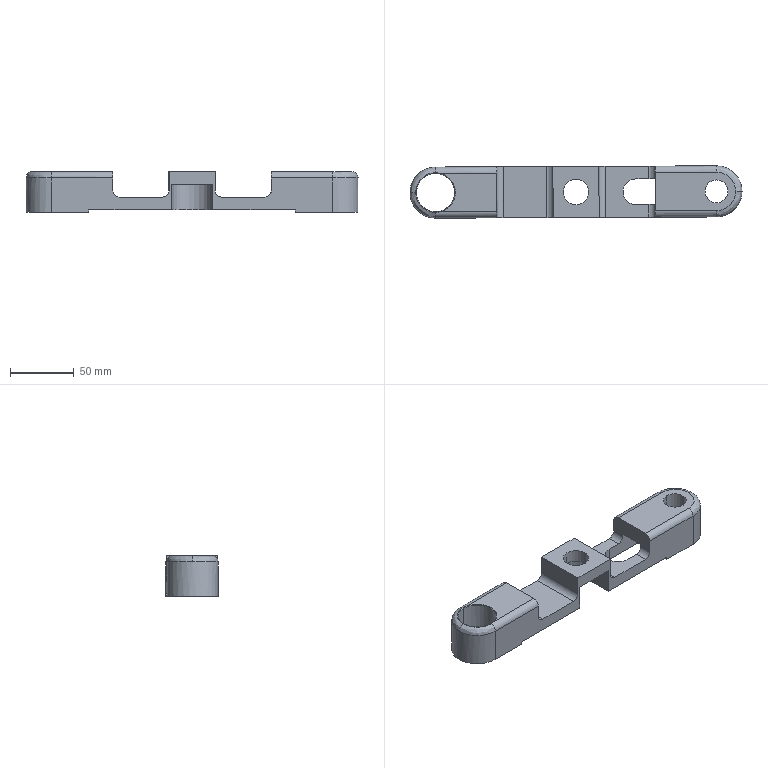Part | SolidWorks | features BaseBody 1 | 1 solid | 64 faces | box 259.998 x 40.957 x 32 mm | volume 152356 mm3 | plane 28 | cylinder 27 | spline 9 | commonest cylinder face diameters 10 x9 34 x5 20 x4 40 x4 18 x2 30 x2